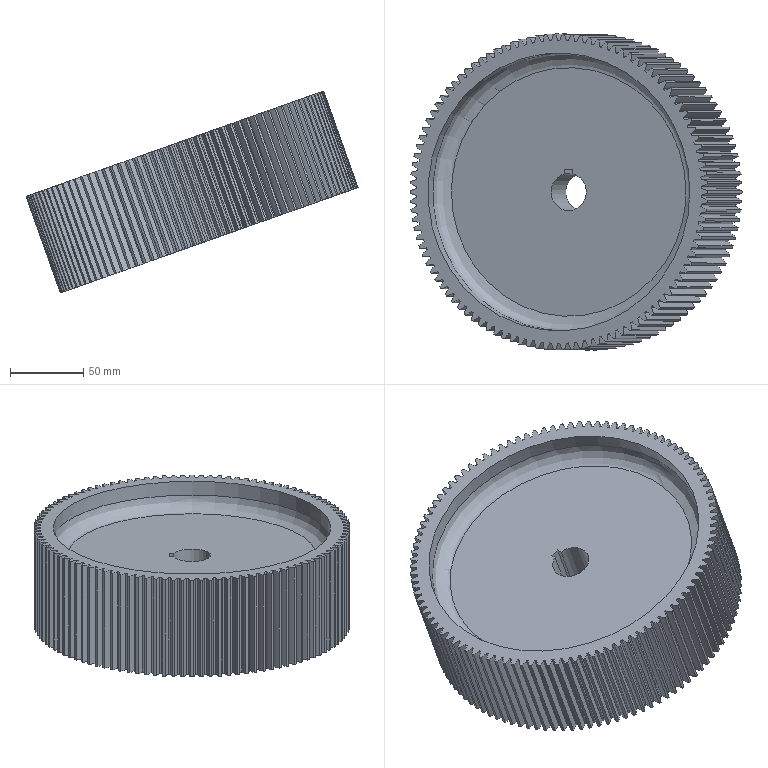Part | STEP file | GEAR1-2_id418_x_t | 1 solid | 436 faces | box 226.977 x 215.948 x 138.087 mm | volume 1339603 mm3 | cylinder 427 | plane 7 | other 2 | commonest cylinder face diameters 70.905 x212 207 x106 216 x106 190 x2 25.5 x1